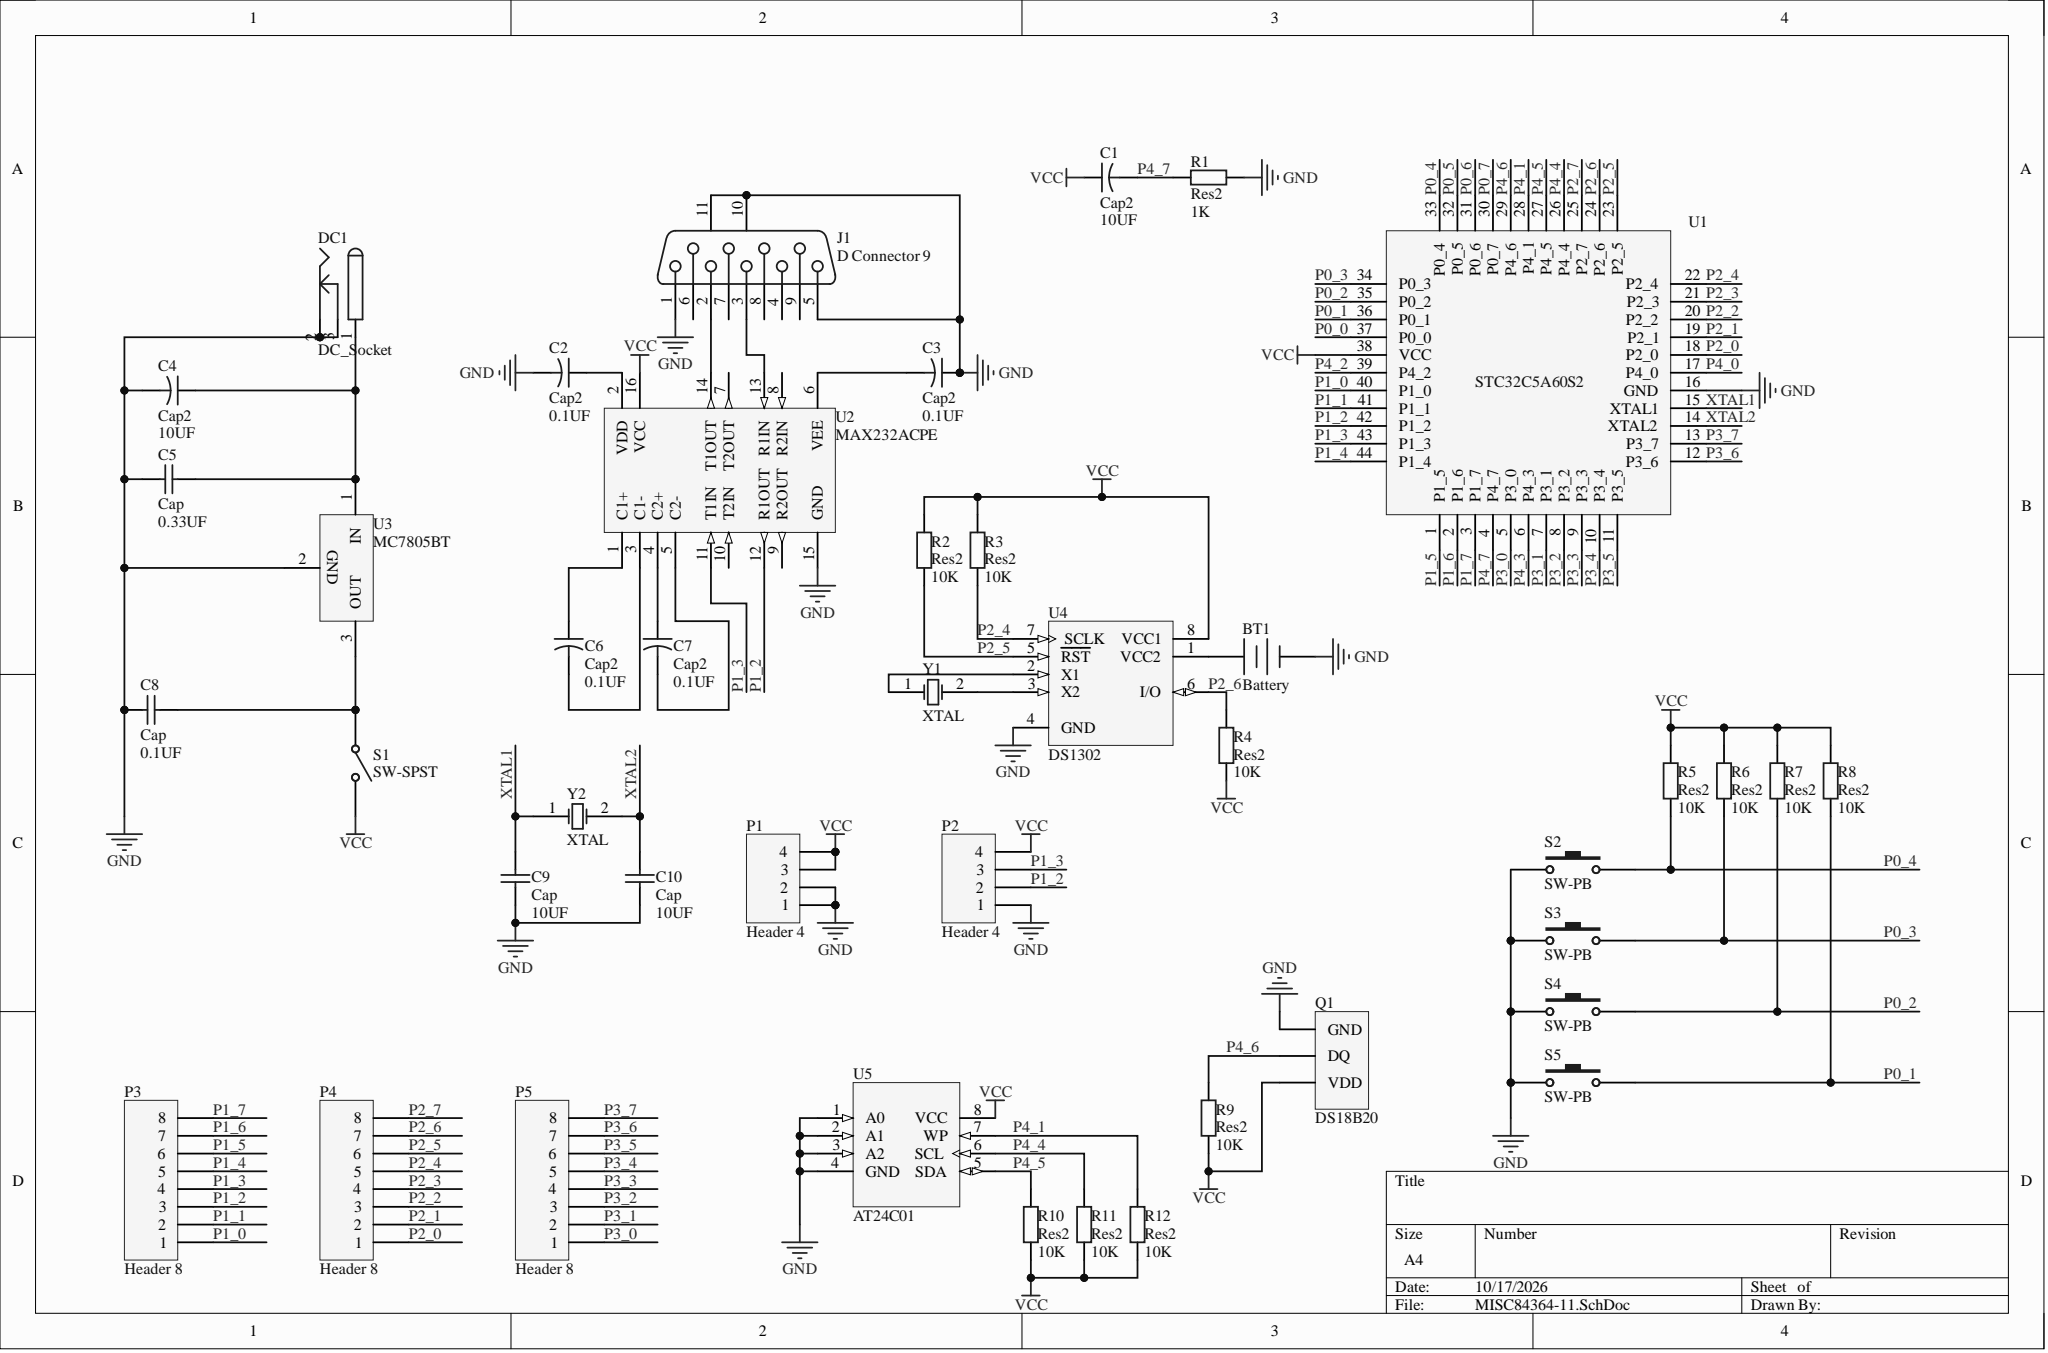Circuit board | Altium Designer | 43 parts | 50 nets
Bill of materials:
Comment,Description,Designator,Footprint,LibRef,Quantity
"Battery","Multicell Battery","BT1","BAT-2","Battery","1"
"Cap2","Capacitor","C1, C2, C3, C4, C6, C7","CAPR5-4X5","Cap2","6"
"Cap","Capacitor","C5, C8, C9, C10","RAD-0.1","Cap","4"
"DC_Socket","","DC1","DC-002","DC_Socket","1"
"D Connector 9","Receptacle Assembly, 9 Position, Right Angle","J1","DSUB1.385-2H9","D Connector 9","1"
"Header 4","Header, 4-Pin","P1, P2","HDR1X4","Header 4","2"
"Header 8","Header, 8-Pin","P3, P4, P5","HDR1X8","Header 8","3"
"DS18B20","","Q1","HDR1X3","DS18B20","1"
"Res2","Resistor","R1, R2, R3, R4, R5, R6, R7, R8, R9, R10, R11, R12","AXIAL-0.4","Res2","12"
"SW-SPST","Single-Pole, Single-Throw Switch","S1","SPST-2","SW-SPST","1"
"SW-PB","Switch","S2, S3, S4, S5","SPST-2","SW-PB","4"
"STC32C5A60S2","STC32C5A60S2","U1","LQFP48 7X7","STC32C5A60S2","1"
"MAX232ACPE","+5V Powered, Multi-Channel RS-232 Driver/Receiver","U2","PE16A","MAX232ACPE","1"
"MC7805BT","3-Terminal Positive Fixed Voltage Regulator","U3","221A-04","MC7805BT","1"
"DS1302","Trickle Charge Timekeeping Chip","U4","DIP8","DS1302","1"
"AT24C01","1Kbit (128 x 8), 2-wire Bus Automotive Serial EEPROM with Write Protect, 2.5V, 8-Pin SOIC, Tape & Reel","U5","DIP-8","AT24C01BN-SP25-T","1"
"XTAL","Crystal Oscillator","Y1, Y2","R38","XTAL","2"
Netlist (Protel format):
[
BT1
BAT-2
Battery



]
[
C1
CAPR5-4X5
Cap2



]
[
C2
CAPR5-4X5
Cap2



]
[
C3
CAPR5-4X5
Cap2



]
[
C4
CAPR5-4X5
Cap2



]
[
C5
RAD-0.1
Cap



]
[
C6
CAPR5-4X5
Cap2



]
[
C7
CAPR5-4X5
Cap2



]
[
C8
RAD-0.1
Cap



]
[
C9
RAD-0.1
Cap



]
[
C10
RAD-0.1
Cap



]
[
DC1
DC-002
DC_Socket



]
[
J1
DSUB1.385-2H9
D Connector 9



]
[
P1
HDR1X4
Header 4



]
[
P2
HDR1X4
Header 4



]
[
P3
HDR1X8
Header 8



]
[
P4
HDR1X8
Header 8



]
[
P5
HDR1X8
Header 8



]
[
Q1
HDR1X3
DS18B20



]
[
R1
AXIAL-0.4
Res2



]
[
R2
AXIAL-0.4
Res2



]
[
R3
AXIAL-0.4
Res2



]
[
R4
AXIAL-0.4
Res2



]
[
R5
AXIAL-0.4
Res2



]
[
R6
AXIAL-0.4
Res2



]
[
R7
AXIAL-0.4
Res2



]
[
R8
AXIAL-0.4
Res2



]
[
R9
AXIAL-0.4
Res2



]
[
R10
AXIAL-0.4
Res2



]
[
R11
AXIAL-0.4
Res2



]
[
R12
AXIAL-0.4
Res2



]
[
S1
SPST-2
SW-SPST



]
[
S2
SPST-2
SW-PB



]
[
S3
SPST-2
SW-PB



]
[
S4
SPST-2
SW-PB



]
[
S5
SPST-2
SW-PB



]
[
U1
LQFP48 7X7
STC32C5A60S2



]
[
U2
PE16A
MAX232ACPE



]
[
U3
221A-04
MC7805BT



]
[
U4
DIP8
DS1302



]
[
U5
DIP-8
AT24C01



]
[
Y1
R38
XTAL



]
[
Y2
R38
XTAL



]
(
XTAL2
C10-2
U1-14
Y2-2
)
(
XTAL1
C9-2
U1-15
Y2-1
)
(
VCC
C1-1
P1-3
P1-4
P2-4
Q1-3
R2-2
R3-2
R4-1
R5-2
R6-2
R7-2
R8-2
R9-1
R10-1
R11-1
R12-1
S1-2
U1-38
U2-16
U4-8
U5-8
)
(
P4_7
C1-2
R1-2
U1-4
)
(
P4_6
Q1-2
R9-2
U1-29
)
(
P4_5
R10-2
U1-27
U5-5
)
(
P4_4
R11-2
U1-26
U5-6
)
(
P4_1
R12-2
U1-28
U5-7
)
(
P3_7
P5-8
U1-13
)
(
P3_6
P5-7
U1-12
)
(
P3_5
P5-6
U1-11
)
(
P3_4
P5-5
U1-10
)
(
P3_3
P5-4
U1-9
)
(
P3_2
P5-3
U1-8
)
(
P3_1
P5-2
U1-7
)
(
P3_0
P5-1
U1-5
)
(
P2_7
P4-8
U1-25
)
(
P2_6
P4-7
R4-2
U1-24
U4-6
)
(
P2_5
P4-6
R2-1
U1-23
U4-5
)
(
P2_4
P4-5
R3-1
U1-22
U4-7
)
(
P2_3
P4-4
U1-21
)
(
P2_2
P4-3
U1-20
)
(
P2_1
P4-2
U1-19
)
(
P2_0
P4-1
U1-18
)
(
P1_7
P3-8
U1-3
)
(
P1_6
P3-7
U1-2
)
(
P1_5
P3-6
U1-1
)
(
P1_4
P3-5
U1-44
)
(
P1_3
P2-3
P3-4
U1-43
U2-11
)
(
P1_2
P2-2
P3-3
U1-42
U2-12
)
(
P1_1
P3-2
U1-41
)
(
P1_0
P3-1
U1-40
)
(
P0_4
R5-1
S2-2
U1-33
)
(
P0_3
R6-1
S3-2
U1-34
)
(
P0_2
R7-1
S4-2
U1-35
)
(
P0_1
R8-1
S5-2
U1-36
)
(
NetU4_3
U4-3
Y1-2
)
(
NetU4_2
U4-2
Y1-1
)
(
NetJ1_3
J1-3
U2-13
)
(
NetJ1_2
J1-2
U2-14
)
(
NetC8_2
C8-2
S1-1
U3-3
)
(
NetC7_2
C7-2
U2-5
)
(
NetC7_1
C7-1
U2-4
)
(
NetC6_2
C6-2
U2-3
)
(
NetC6_1
C6-1
U2-1
)
(
NetC4_1
C4-1
C5-2
DC1-1
U3-1
)
(
NetC3_2
C3-2
U2-6
)
(
NetC2_1
C2-1
U2-2
)
(
NetBT1_1
BT1-1
U4-1
)
(
GND
BT1-2
C2-2
C3-1
C4-2
C5-1
C8-1
C9-1
C10-1
DC1-2
DC1-3
J1-1
J1-5
J1-10
J1-11
P1-1
P1-2
P2-1
Q1-1
R1-1
S2-1
S3-1
S4-1
S5-1
U1-16
U2-15
U3-2
U4-4
U5-1
U5-2
U5-3
U5-4
)